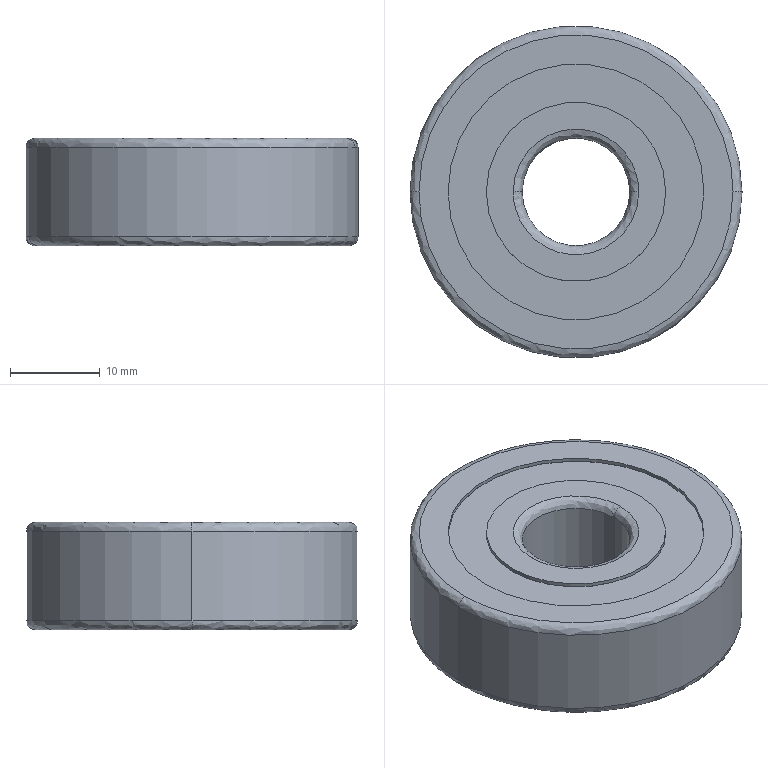Part | SolidWorks | features BaseBody 1 | 1 solid | 96 faces | box 37 x 37 x 12 mm | volume 8313 mm3 | spline 68 | cylinder 20 | plane 8 | commonest cylinder face diameters 20 x8 28.5 x8 12 x2 37 x2